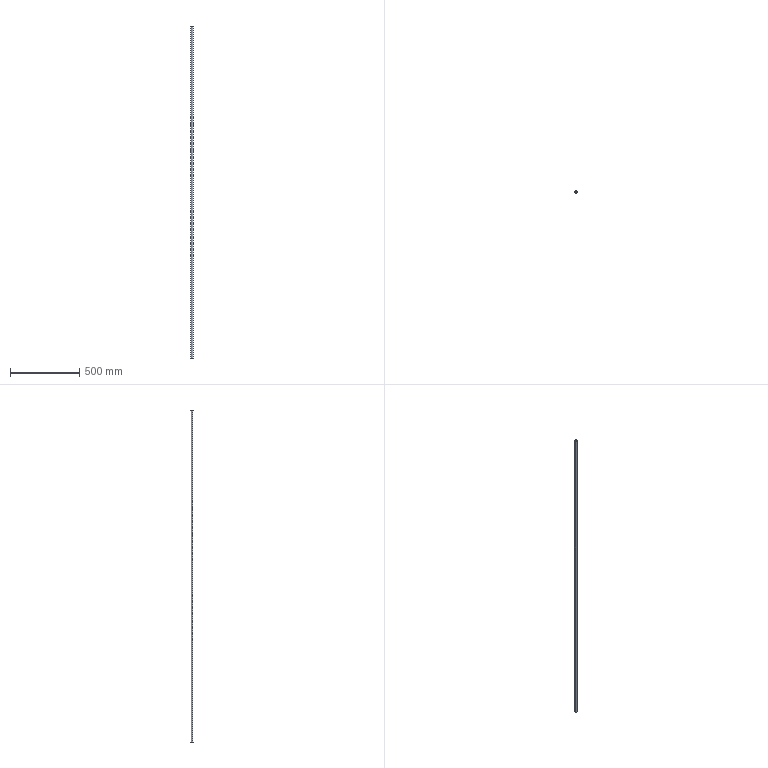Part | STEP file | 1 solid | 6 faces | box 18 x 18 x 2400 mm | volume 292168 mm3 | cylinder 4 | plane 2 | commonest cylinder face diameters 13 x2 18 x2
STEP:
#1=CARTESIAN_POINT('',(0.,0.,0.));
#2=DIRECTION('',(0.,0.,1.));
#3=DIRECTION('',(1.,0.,0.));
#4=AXIS2_PLACEMENT_3D('',#1,#2,#3);
#5=CARTESIAN_POINT('',(-6.5,0.,0.));
#6=VERTEX_POINT('',#5);
#7=CARTESIAN_POINT('',(6.5,0.,0.));
#8=VERTEX_POINT('',#7);
#9=CARTESIAN_POINT('',(0.,0.,0.));
#10=DIRECTION('',(0.,0.,-1.));
#11=DIRECTION('',(-1.,0.,0.));
#12=AXIS2_PLACEMENT_3D('',#9,#10,#11);
#13=CIRCLE('',#12,6.5);
#14=CARTESIAN_POINT('',(0.,0.,2400.));
#15=DIRECTION('',(0.,0.,-1.));
#16=DIRECTION('',(-1.,0.,0.));
#17=AXIS2_PLACEMENT_3D('',#14,#15,#16);
#18=CYLINDRICAL_SURFACE('',#17,6.5);
#19=CARTESIAN_POINT('',(0.,2400.));
#20=DIRECTION('',(1.,0.));
#21=VECTOR('',#20,1.);
#22=LINE('',#19,#21);
#23=(GEOMETRIC_REPRESENTATION_CONTEXT(2)PARAMETRIC_REPRESENTATION_CONTEXT()REPRESENTATION_CONTEXT('',''));
#24=DEFINITIONAL_REPRESENTATION('',(#22),#23);
#25=PCURVE('',#18,#24);
#26=CARTESIAN_POINT('',(0.,0.,0.));
#27=DIRECTION('',(0.,0.,1.));
#28=DIRECTION('',(1.,0.,0.));
#29=AXIS2_PLACEMENT_3D('',#26,#27,#28);
#30=PLANE('',#29);
#31=CARTESIAN_POINT('',(-6.5,0.));
#32=CARTESIAN_POINT('',(-6.5,11.258));
#33=CARTESIAN_POINT('',(3.25,5.629));
#34=CARTESIAN_POINT('',(13.,0.));
#35=CARTESIAN_POINT('',(3.25,-5.629));
#36=CARTESIAN_POINT('',(-6.5,-11.258));
#37=CARTESIAN_POINT('',(-6.5,0.));
#38=(BOUNDED_CURVE()B_SPLINE_CURVE(2,(#31,#32,#33,#34,#35,#36,#37),.UNSPECIFIED.,.T.,.F.)B_SPLINE_CURVE_WITH_KNOTS((1,2,2,2,2,1),(-2.094,0.,2.094,4.189,6.283,8.378),.UNSPECIFIED.)CURVE()GEOMETRIC_REPRESENTATION_ITEM()RATIONAL_B_SPLINE_CURVE((1.,0.5,1.,0.5,1.,0.5,1.))REPRESENTATION_ITEM(''));
#39=(GEOMETRIC_REPRESENTATION_CONTEXT(2)PARAMETRIC_REPRESENTATION_CONTEXT()REPRESENTATION_CONTEXT('',''));
#40=DEFINITIONAL_REPRESENTATION('',(#38),#39);
#41=PCURVE('',#30,#40);
#42=SURFACE_CURVE('',#13,(#25,#41),.PCURVE_S1.);
#43=EDGE_CURVE('',#6,#8,#42,.T.);
#44=ORIENTED_EDGE('',*,*,#43,.F.);
#45=CARTESIAN_POINT('',(-6.5,0.,2400.));
#46=VERTEX_POINT('',#45);
#47=CARTESIAN_POINT('',(-6.5,0.,2400.));
#48=DIRECTION('',(0.,0.,-1.));
#49=VECTOR('',#48,1.);
#50=LINE('',#47,#49);
#51=CARTESIAN_POINT('',(0.,0.));
#52=DIRECTION('',(0.,1.));
#53=VECTOR('',#52,1.);
#54=LINE('',#51,#53);
#55=(GEOMETRIC_REPRESENTATION_CONTEXT(2)PARAMETRIC_REPRESENTATION_CONTEXT()REPRESENTATION_CONTEXT('',''));
#56=DEFINITIONAL_REPRESENTATION('',(#54),#55);
#57=PCURVE('',#18,#56);
#58=CARTESIAN_POINT('',(0.,0.,2400.));
#59=DIRECTION('',(0.,0.,-1.));
#60=DIRECTION('',(-1.,0.,0.));
#61=AXIS2_PLACEMENT_3D('',#58,#59,#60);
#62=CYLINDRICAL_SURFACE('',#61,6.5);
#63=CARTESIAN_POINT('',(6.283,0.));
#64=DIRECTION('',(0.,1.));
#65=VECTOR('',#64,1.);
#66=LINE('',#63,#65);
#67=(GEOMETRIC_REPRESENTATION_CONTEXT(2)PARAMETRIC_REPRESENTATION_CONTEXT()REPRESENTATION_CONTEXT('',''));
#68=DEFINITIONAL_REPRESENTATION('',(#66),#67);
#69=PCURVE('',#62,#68);
#70=SURFACE_CURVE('',#50,(#57,#69),.PCURVE_S1.);
#71=EDGE_CURVE('',#46,#6,#70,.T.);
#72=ORIENTED_EDGE('',*,*,#71,.F.);
#73=CARTESIAN_POINT('',(6.5,0.,2400.));
#74=VERTEX_POINT('',#73);
#75=CARTESIAN_POINT('',(0.,0.,2400.));
#76=DIRECTION('',(0.,0.,-1.));
#77=DIRECTION('',(-1.,0.,0.));
#78=AXIS2_PLACEMENT_3D('',#75,#76,#77);
#79=CIRCLE('',#78,6.5);
#80=CARTESIAN_POINT('',(0.,0.));
#81=DIRECTION('',(1.,0.));
#82=VECTOR('',#81,1.);
#83=LINE('',#80,#82);
#84=(GEOMETRIC_REPRESENTATION_CONTEXT(2)PARAMETRIC_REPRESENTATION_CONTEXT()REPRESENTATION_CONTEXT('',''));
#85=DEFINITIONAL_REPRESENTATION('',(#83),#84);
#86=PCURVE('',#18,#85);
#87=CARTESIAN_POINT('',(0.,0.,2400.));
#88=DIRECTION('',(0.,0.,1.));
#89=DIRECTION('',(1.,0.,0.));
#90=AXIS2_PLACEMENT_3D('',#87,#88,#89);
#91=PLANE('',#90);
#92=CARTESIAN_POINT('',(-6.5,0.));
#93=CARTESIAN_POINT('',(-6.5,11.258));
#94=CARTESIAN_POINT('',(3.25,5.629));
#95=CARTESIAN_POINT('',(13.,0.));
#96=CARTESIAN_POINT('',(3.25,-5.629));
#97=CARTESIAN_POINT('',(-6.5,-11.258));
#98=CARTESIAN_POINT('',(-6.5,0.));
#99=(BOUNDED_CURVE()B_SPLINE_CURVE(2,(#92,#93,#94,#95,#96,#97,#98),.UNSPECIFIED.,.T.,.F.)B_SPLINE_CURVE_WITH_KNOTS((1,2,2,2,2,1),(-2.094,0.,2.094,4.189,6.283,8.378),.UNSPECIFIED.)CURVE()GEOMETRIC_REPRESENTATION_ITEM()RATIONAL_B_SPLINE_CURVE((1.,0.5,1.,0.5,1.,0.5,1.))REPRESENTATION_ITEM(''));
#100=(GEOMETRIC_REPRESENTATION_CONTEXT(2)PARAMETRIC_REPRESENTATION_CONTEXT()REPRESENTATION_CONTEXT('',''));
#101=DEFINITIONAL_REPRESENTATION('',(#99),#100);
#102=PCURVE('',#91,#101);
#103=SURFACE_CURVE('',#79,(#86,#102),.PCURVE_S1.);
#104=EDGE_CURVE('',#46,#74,#103,.T.);
#105=ORIENTED_EDGE('',*,*,#104,.T.);
#106=CARTESIAN_POINT('',(6.5,0.,2400.));
#107=DIRECTION('',(0.,0.,-1.));
#108=VECTOR('',#107,1.);
#109=LINE('',#106,#108);
#110=CARTESIAN_POINT('',(3.142,0.));
#111=DIRECTION('',(0.,1.));
#112=VECTOR('',#111,1.);
#113=LINE('',#110,#112);
#114=(GEOMETRIC_REPRESENTATION_CONTEXT(2)PARAMETRIC_REPRESENTATION_CONTEXT()REPRESENTATION_CONTEXT('',''));
#115=DEFINITIONAL_REPRESENTATION('',(#113),#114);
#116=PCURVE('',#18,#115);
#117=CARTESIAN_POINT('',(3.142,0.));
#118=DIRECTION('',(0.,1.));
#119=VECTOR('',#118,1.);
#120=LINE('',#117,#119);
#121=(GEOMETRIC_REPRESENTATION_CONTEXT(2)PARAMETRIC_REPRESENTATION_CONTEXT()REPRESENTATION_CONTEXT('',''));
#122=DEFINITIONAL_REPRESENTATION('',(#120),#121);
#123=PCURVE('',#62,#122);
#124=SURFACE_CURVE('',#109,(#116,#123),.PCURVE_S1.);
#125=EDGE_CURVE('',#74,#8,#124,.T.);
#126=ORIENTED_EDGE('',*,*,#125,.T.);
#127=EDGE_LOOP('',(#44,#72,#105,#126));
#128=FACE_BOUND('',#127,.F.);
#129=ADVANCED_FACE('',(#128),#18,.F.);
#130=ORIENTED_EDGE('',*,*,#104,.T.);
#131=CARTESIAN_POINT('',(0.,0.,2400.));
#132=DIRECTION('',(0.,0.,-1.));
#133=DIRECTION('',(-1.,0.,0.));
#134=AXIS2_PLACEMENT_3D('',#131,#132,#133);
#135=CIRCLE('',#134,6.5);
#136=CARTESIAN_POINT('',(-6.5,0.));
#137=CARTESIAN_POINT('',(-6.5,11.258));
#138=CARTESIAN_POINT('',(3.25,5.629));
#139=CARTESIAN_POINT('',(13.,0.));
#140=CARTESIAN_POINT('',(3.25,-5.629));
#141=CARTESIAN_POINT('',(-6.5,-11.258));
#142=CARTESIAN_POINT('',(-6.5,0.));
#143=(BOUNDED_CURVE()B_SPLINE_CURVE(2,(#136,#137,#138,#139,#140,#141,#142),.UNSPECIFIED.,.T.,.F.)B_SPLINE_CURVE_WITH_KNOTS((1,2,2,2,2,1),(-2.094,0.,2.094,4.189,6.283,8.378),.UNSPECIFIED.)CURVE()GEOMETRIC_REPRESENTATION_ITEM()RATIONAL_B_SPLINE_CURVE((1.,0.5,1.,0.5,1.,0.5,1.))REPRESENTATION_ITEM(''));
#144=(GEOMETRIC_REPRESENTATION_CONTEXT(2)PARAMETRIC_REPRESENTATION_CONTEXT()REPRESENTATION_CONTEXT('',''));
#145=DEFINITIONAL_REPRESENTATION('',(#143),#144);
#146=PCURVE('',#91,#145);
#147=CARTESIAN_POINT('',(0.,0.));
#148=DIRECTION('',(1.,0.));
#149=VECTOR('',#148,1.);
#150=LINE('',#147,#149);
#151=(GEOMETRIC_REPRESENTATION_CONTEXT(2)PARAMETRIC_REPRESENTATION_CONTEXT()REPRESENTATION_CONTEXT('',''));
#152=DEFINITIONAL_REPRESENTATION('',(#150),#151);
#153=PCURVE('',#62,#152);
#154=SURFACE_CURVE('',#135,(#146,#153),.PCURVE_S1.);
#155=EDGE_CURVE('',#74,#46,#154,.T.);
#156=ORIENTED_EDGE('',*,*,#155,.T.);
#157=EDGE_LOOP('',(#130,#156));
#158=FACE_BOUND('',#157,.T.);
#159=CARTESIAN_POINT('',(-9.,0.,2400.));
#160=VERTEX_POINT('',#159);
#161=CARTESIAN_POINT('',(9.,0.,2400.));
#162=VERTEX_POINT('',#161);
#163=CARTESIAN_POINT('',(0.,0.,2400.));
#164=DIRECTION('',(0.,0.,-1.));
#165=DIRECTION('',(-1.,0.,0.));
#166=AXIS2_PLACEMENT_3D('',#163,#164,#165);
#167=CIRCLE('',#166,9.);
#168=CARTESIAN_POINT('',(-9.,0.));
#169=CARTESIAN_POINT('',(-9.,15.588));
#170=CARTESIAN_POINT('',(4.5,7.794));
#171=CARTESIAN_POINT('',(18.,0.));
#172=CARTESIAN_POINT('',(4.5,-7.794));
#173=CARTESIAN_POINT('',(-9.,-15.588));
#174=CARTESIAN_POINT('',(-9.,0.));
#175=(BOUNDED_CURVE()B_SPLINE_CURVE(2,(#168,#169,#170,#171,#172,#173,#174),.UNSPECIFIED.,.T.,.F.)B_SPLINE_CURVE_WITH_KNOTS((1,2,2,2,2,1),(-2.094,0.,2.094,4.189,6.283,8.378),.UNSPECIFIED.)CURVE()GEOMETRIC_REPRESENTATION_ITEM()RATIONAL_B_SPLINE_CURVE((1.,0.5,1.,0.5,1.,0.5,1.))REPRESENTATION_ITEM(''));
#176=(GEOMETRIC_REPRESENTATION_CONTEXT(2)PARAMETRIC_REPRESENTATION_CONTEXT()REPRESENTATION_CONTEXT('',''));
#177=DEFINITIONAL_REPRESENTATION('',(#175),#176);
#178=PCURVE('',#91,#177);
#179=CARTESIAN_POINT('',(0.,0.,2400.));
#180=DIRECTION('',(0.,0.,-1.));
#181=DIRECTION('',(-1.,0.,0.));
#182=AXIS2_PLACEMENT_3D('',#179,#180,#181);
#183=CYLINDRICAL_SURFACE('',#182,9.);
#184=CARTESIAN_POINT('',(0.,0.));
#185=DIRECTION('',(1.,0.));
#186=VECTOR('',#185,1.);
#187=LINE('',#184,#186);
#188=(GEOMETRIC_REPRESENTATION_CONTEXT(2)PARAMETRIC_REPRESENTATION_CONTEXT()REPRESENTATION_CONTEXT('',''));
#189=DEFINITIONAL_REPRESENTATION('',(#187),#188);
#190=PCURVE('',#183,#189);
#191=SURFACE_CURVE('',#167,(#178,#190),.PCURVE_S1.);
#192=EDGE_CURVE('',#160,#162,#191,.T.);
#193=ORIENTED_EDGE('',*,*,#192,.F.);
#194=CARTESIAN_POINT('',(0.,0.,2400.));
#195=DIRECTION('',(0.,0.,-1.));
#196=DIRECTION('',(-1.,0.,0.));
#197=AXIS2_PLACEMENT_3D('',#194,#195,#196);
#198=CIRCLE('',#197,9.);
#199=CARTESIAN_POINT('',(-9.,0.));
#200=CARTESIAN_POINT('',(-9.,15.588));
#201=CARTESIAN_POINT('',(4.5,7.794));
#202=CARTESIAN_POINT('',(18.,0.));
#203=CARTESIAN_POINT('',(4.5,-7.794));
#204=CARTESIAN_POINT('',(-9.,-15.588));
#205=CARTESIAN_POINT('',(-9.,0.));
#206=(BOUNDED_CURVE()B_SPLINE_CURVE(2,(#199,#200,#201,#202,#203,#204,#205),.UNSPECIFIED.,.T.,.F.)B_SPLINE_CURVE_WITH_KNOTS((1,2,2,2,2,1),(-2.094,0.,2.094,4.189,6.283,8.378),.UNSPECIFIED.)CURVE()GEOMETRIC_REPRESENTATION_ITEM()RATIONAL_B_SPLINE_CURVE((1.,0.5,1.,0.5,1.,0.5,1.))REPRESENTATION_ITEM(''));
#207=(GEOMETRIC_REPRESENTATION_CONTEXT(2)PARAMETRIC_REPRESENTATION_CONTEXT()REPRESENTATION_CONTEXT('',''));
#208=DEFINITIONAL_REPRESENTATION('',(#206),#207);
#209=PCURVE('',#91,#208);
#210=CARTESIAN_POINT('',(0.,0.,2400.));
#211=DIRECTION('',(0.,0.,-1.));
#212=DIRECTION('',(-1.,0.,0.));
#213=AXIS2_PLACEMENT_3D('',#210,#211,#212);
#214=CYLINDRICAL_SURFACE('',#213,9.);
#215=CARTESIAN_POINT('',(0.,0.));
#216=DIRECTION('',(1.,0.));
#217=VECTOR('',#216,1.);
#218=LINE('',#215,#217);
#219=(GEOMETRIC_REPRESENTATION_CONTEXT(2)PARAMETRIC_REPRESENTATION_CONTEXT()REPRESENTATION_CONTEXT('',''));
#220=DEFINITIONAL_REPRESENTATION('',(#218),#219);
#221=PCURVE('',#214,#220);
#222=SURFACE_CURVE('',#198,(#209,#221),.PCURVE_S1.);
#223=EDGE_CURVE('',#162,#160,#222,.T.);
#224=ORIENTED_EDGE('',*,*,#223,.F.);
#225=EDGE_LOOP('',(#193,#224));
#226=FACE_BOUND('',#225,.T.);
#227=ADVANCED_FACE('',(#158,#226),#91,.T.);
#228=ORIENTED_EDGE('',*,*,#43,.F.);
#229=CARTESIAN_POINT('',(0.,0.,0.));
#230=DIRECTION('',(0.,0.,-1.));
#231=DIRECTION('',(-1.,0.,0.));
#232=AXIS2_PLACEMENT_3D('',#229,#230,#231);
#233=CIRCLE('',#232,6.5);
#234=CARTESIAN_POINT('',(-6.5,0.));
#235=CARTESIAN_POINT('',(-6.5,11.258));
#236=CARTESIAN_POINT('',(3.25,5.629));
#237=CARTESIAN_POINT('',(13.,0.));
#238=CARTESIAN_POINT('',(3.25,-5.629));
#239=CARTESIAN_POINT('',(-6.5,-11.258));
#240=CARTESIAN_POINT('',(-6.5,0.));
#241=(BOUNDED_CURVE()B_SPLINE_CURVE(2,(#234,#235,#236,#237,#238,#239,#240),.UNSPECIFIED.,.T.,.F.)B_SPLINE_CURVE_WITH_KNOTS((1,2,2,2,2,1),(-2.094,0.,2.094,4.189,6.283,8.378),.UNSPECIFIED.)CURVE()GEOMETRIC_REPRESENTATION_ITEM()RATIONAL_B_SPLINE_CURVE((1.,0.5,1.,0.5,1.,0.5,1.))REPRESENTATION_ITEM(''));
#242=(GEOMETRIC_REPRESENTATION_CONTEXT(2)PARAMETRIC_REPRESENTATION_CONTEXT()REPRESENTATION_CONTEXT('',''));
#243=DEFINITIONAL_REPRESENTATION('',(#241),#242);
#244=PCURVE('',#30,#243);
#245=CARTESIAN_POINT('',(0.,2400.));
#246=DIRECTION('',(1.,0.));
#247=VECTOR('',#246,1.);
#248=LINE('',#245,#247);
#249=(GEOMETRIC_REPRESENTATION_CONTEXT(2)PARAMETRIC_REPRESENTATION_CONTEXT()REPRESENTATION_CONTEXT('',''));
#250=DEFINITIONAL_REPRESENTATION('',(#248),#249);
#251=PCURVE('',#62,#250);
#252=SURFACE_CURVE('',#233,(#244,#251),.PCURVE_S1.);
#253=EDGE_CURVE('',#8,#6,#252,.T.);
#254=ORIENTED_EDGE('',*,*,#253,.F.);
#255=EDGE_LOOP('',(#228,#254));
#256=FACE_BOUND('',#255,.T.);
#257=CARTESIAN_POINT('',(-9.,0.,0.));
#258=VERTEX_POINT('',#257);
#259=CARTESIAN_POINT('',(9.,0.,0.));
#260=VERTEX_POINT('',#259);
#261=CARTESIAN_POINT('',(0.,0.,0.));
#262=DIRECTION('',(0.,0.,1.));
#263=DIRECTION('',(-1.,0.,0.));
#264=AXIS2_PLACEMENT_3D('',#261,#262,#263);
#265=CIRCLE('',#264,9.);
#266=CARTESIAN_POINT('',(0.,0.));
#267=DIRECTION('',(-1.,0.));
#268=AXIS2_PLACEMENT_2D('',#266,#267);
#269=CIRCLE('',#268,9.);
#270=(GEOMETRIC_REPRESENTATION_CONTEXT(2)PARAMETRIC_REPRESENTATION_CONTEXT()REPRESENTATION_CONTEXT('',''));
#271=DEFINITIONAL_REPRESENTATION('',(#269),#270);
#272=PCURVE('',#30,#271);
#273=CARTESIAN_POINT('',(6.283,2400.));
#274=DIRECTION('',(-1.,0.));
#275=VECTOR('',#274,1.);
#276=LINE('',#273,#275);
#277=(GEOMETRIC_REPRESENTATION_CONTEXT(2)PARAMETRIC_REPRESENTATION_CONTEXT()REPRESENTATION_CONTEXT('',''));
#278=DEFINITIONAL_REPRESENTATION('',(#276),#277);
#279=PCURVE('',#214,#278);
#280=SURFACE_CURVE('',#265,(#272,#279),.PCURVE_S1.);
#281=EDGE_CURVE('',#258,#260,#280,.T.);
#282=ORIENTED_EDGE('',*,*,#281,.F.);
#283=CARTESIAN_POINT('',(0.,0.,0.));
#284=DIRECTION('',(0.,0.,1.));
#285=DIRECTION('',(-1.,0.,0.));
#286=AXIS2_PLACEMENT_3D('',#283,#284,#285);
#287=CIRCLE('',#286,9.);
#288=CARTESIAN_POINT('',(0.,0.));
#289=DIRECTION('',(-1.,0.));
#290=AXIS2_PLACEMENT_2D('',#288,#289);
#291=CIRCLE('',#290,9.);
#292=(GEOMETRIC_REPRESENTATION_CONTEXT(2)PARAMETRIC_REPRESENTATION_CONTEXT()REPRESENTATION_CONTEXT('',''));
#293=DEFINITIONAL_REPRESENTATION('',(#291),#292);
#294=PCURVE('',#30,#293);
#295=CARTESIAN_POINT('',(6.283,2400.));
#296=DIRECTION('',(-1.,0.));
#297=VECTOR('',#296,1.);
#298=LINE('',#295,#297);
#299=(GEOMETRIC_REPRESENTATION_CONTEXT(2)PARAMETRIC_REPRESENTATION_CONTEXT()REPRESENTATION_CONTEXT('',''));
#300=DEFINITIONAL_REPRESENTATION('',(#298),#299);
#301=PCURVE('',#183,#300);
#302=SURFACE_CURVE('',#287,(#294,#301),.PCURVE_S1.);
#303=EDGE_CURVE('',#260,#258,#302,.T.);
#304=ORIENTED_EDGE('',*,*,#303,.F.);
#305=EDGE_LOOP('',(#282,#304));
#306=FACE_BOUND('',#305,.T.);
#307=ADVANCED_FACE('',(#256,#306),#30,.F.);
#308=CARTESIAN_POINT('',(9.,0.,2400.));
#309=DIRECTION('',(0.,0.,-1.));
#310=VECTOR('',#309,1.);
#311=LINE('',#308,#310);
#312=CARTESIAN_POINT('',(3.142,0.));
#313=DIRECTION('',(0.,1.));
#314=VECTOR('',#313,1.);
#315=LINE('',#312,#314);
#316=(GEOMETRIC_REPRESENTATION_CONTEXT(2)PARAMETRIC_REPRESENTATION_CONTEXT()REPRESENTATION_CONTEXT('',''));
#317=DEFINITIONAL_REPRESENTATION('',(#315),#316);
#318=PCURVE('',#214,#317);
#319=CARTESIAN_POINT('',(3.142,0.));
#320=DIRECTION('',(0.,1.));
#321=VECTOR('',#320,1.);
#322=LINE('',#319,#321);
#323=(GEOMETRIC_REPRESENTATION_CONTEXT(2)PARAMETRIC_REPRESENTATION_CONTEXT()REPRESENTATION_CONTEXT('',''));
#324=DEFINITIONAL_REPRESENTATION('',(#322),#323);
#325=PCURVE('',#183,#324);
#326=SURFACE_CURVE('',#311,(#318,#325),.PCURVE_S1.);
#327=EDGE_CURVE('',#162,#260,#326,.T.);
#328=ORIENTED_EDGE('',*,*,#327,.F.);
#329=ORIENTED_EDGE('',*,*,#223,.T.);
#330=CARTESIAN_POINT('',(-9.,0.,2400.));
#331=DIRECTION('',(0.,0.,-1.));
#332=VECTOR('',#331,1.);
#333=LINE('',#330,#332);
#334=CARTESIAN_POINT('',(6.283,0.));
#335=DIRECTION('',(0.,1.));
#336=VECTOR('',#335,1.);
#337=LINE('',#334,#336);
#338=(GEOMETRIC_REPRESENTATION_CONTEXT(2)PARAMETRIC_REPRESENTATION_CONTEXT()REPRESENTATION_CONTEXT('',''));
#339=DEFINITIONAL_REPRESENTATION('',(#337),#338);
#340=PCURVE('',#214,#339);
#341=CARTESIAN_POINT('',(0.,0.));
#342=DIRECTION('',(0.,1.));
#343=VECTOR('',#342,1.);
#344=LINE('',#341,#343);
#345=(GEOMETRIC_REPRESENTATION_CONTEXT(2)PARAMETRIC_REPRESENTATION_CONTEXT()REPRESENTATION_CONTEXT('',''));
#346=DEFINITIONAL_REPRESENTATION('',(#344),#345);
#347=PCURVE('',#183,#346);
#348=SURFACE_CURVE('',#333,(#340,#347),.PCURVE_S1.);
#349=EDGE_CURVE('',#160,#258,#348,.T.);
#350=ORIENTED_EDGE('',*,*,#349,.T.);
#351=ORIENTED_EDGE('',*,*,#281,.T.);
#352=EDGE_LOOP('',(#328,#329,#350,#351));
#353=FACE_BOUND('',#352,.T.);
#354=ADVANCED_FACE('',(#353),#214,.T.);
#355=ORIENTED_EDGE('',*,*,#71,.T.);
#356=ORIENTED_EDGE('',*,*,#253,.F.);
#357=ORIENTED_EDGE('',*,*,#125,.F.);
#358=ORIENTED_EDGE('',*,*,#155,.T.);
#359=EDGE_LOOP('',(#355,#356,#357,#358));
#360=FACE_BOUND('',#359,.F.);
#361=ADVANCED_FACE('',(#360),#62,.F.);
#362=ORIENTED_EDGE('',*,*,#192,.T.);
#363=ORIENTED_EDGE('',*,*,#327,.T.);
#364=ORIENTED_EDGE('',*,*,#303,.T.);
#365=ORIENTED_EDGE('',*,*,#349,.F.);
#366=EDGE_LOOP('',(#362,#363,#364,#365));
#367=FACE_BOUND('',#366,.T.);
#368=ADVANCED_FACE('',(#367),#183,.T.);
#369=CLOSED_SHELL('',(#129,#227,#307,#354,#361,#368));
#370=MANIFOLD_SOLID_BREP('',#369);
#371=(LENGTH_UNIT()NAMED_UNIT(*)SI_UNIT(.MILLI.,.METRE.));
#372=UNCERTAINTY_MEASURE_WITH_UNIT(LENGTH_MEASURE(0.0000001),#371,'','');
#373=(NAMED_UNIT(*)PLANE_ANGLE_UNIT()SI_UNIT($,.RADIAN.));
#374=(NAMED_UNIT(*)SI_UNIT($,.STERADIAN.)SOLID_ANGLE_UNIT());
#375=(GEOMETRIC_REPRESENTATION_CONTEXT(3)GLOBAL_UNCERTAINTY_ASSIGNED_CONTEXT((#372))GLOBAL_UNIT_ASSIGNED_CONTEXT((#371,#373,#374))REPRESENTATION_CONTEXT('',''));
#376=ADVANCED_BREP_SHAPE_REPRESENTATION('',(#4,#370),#375);